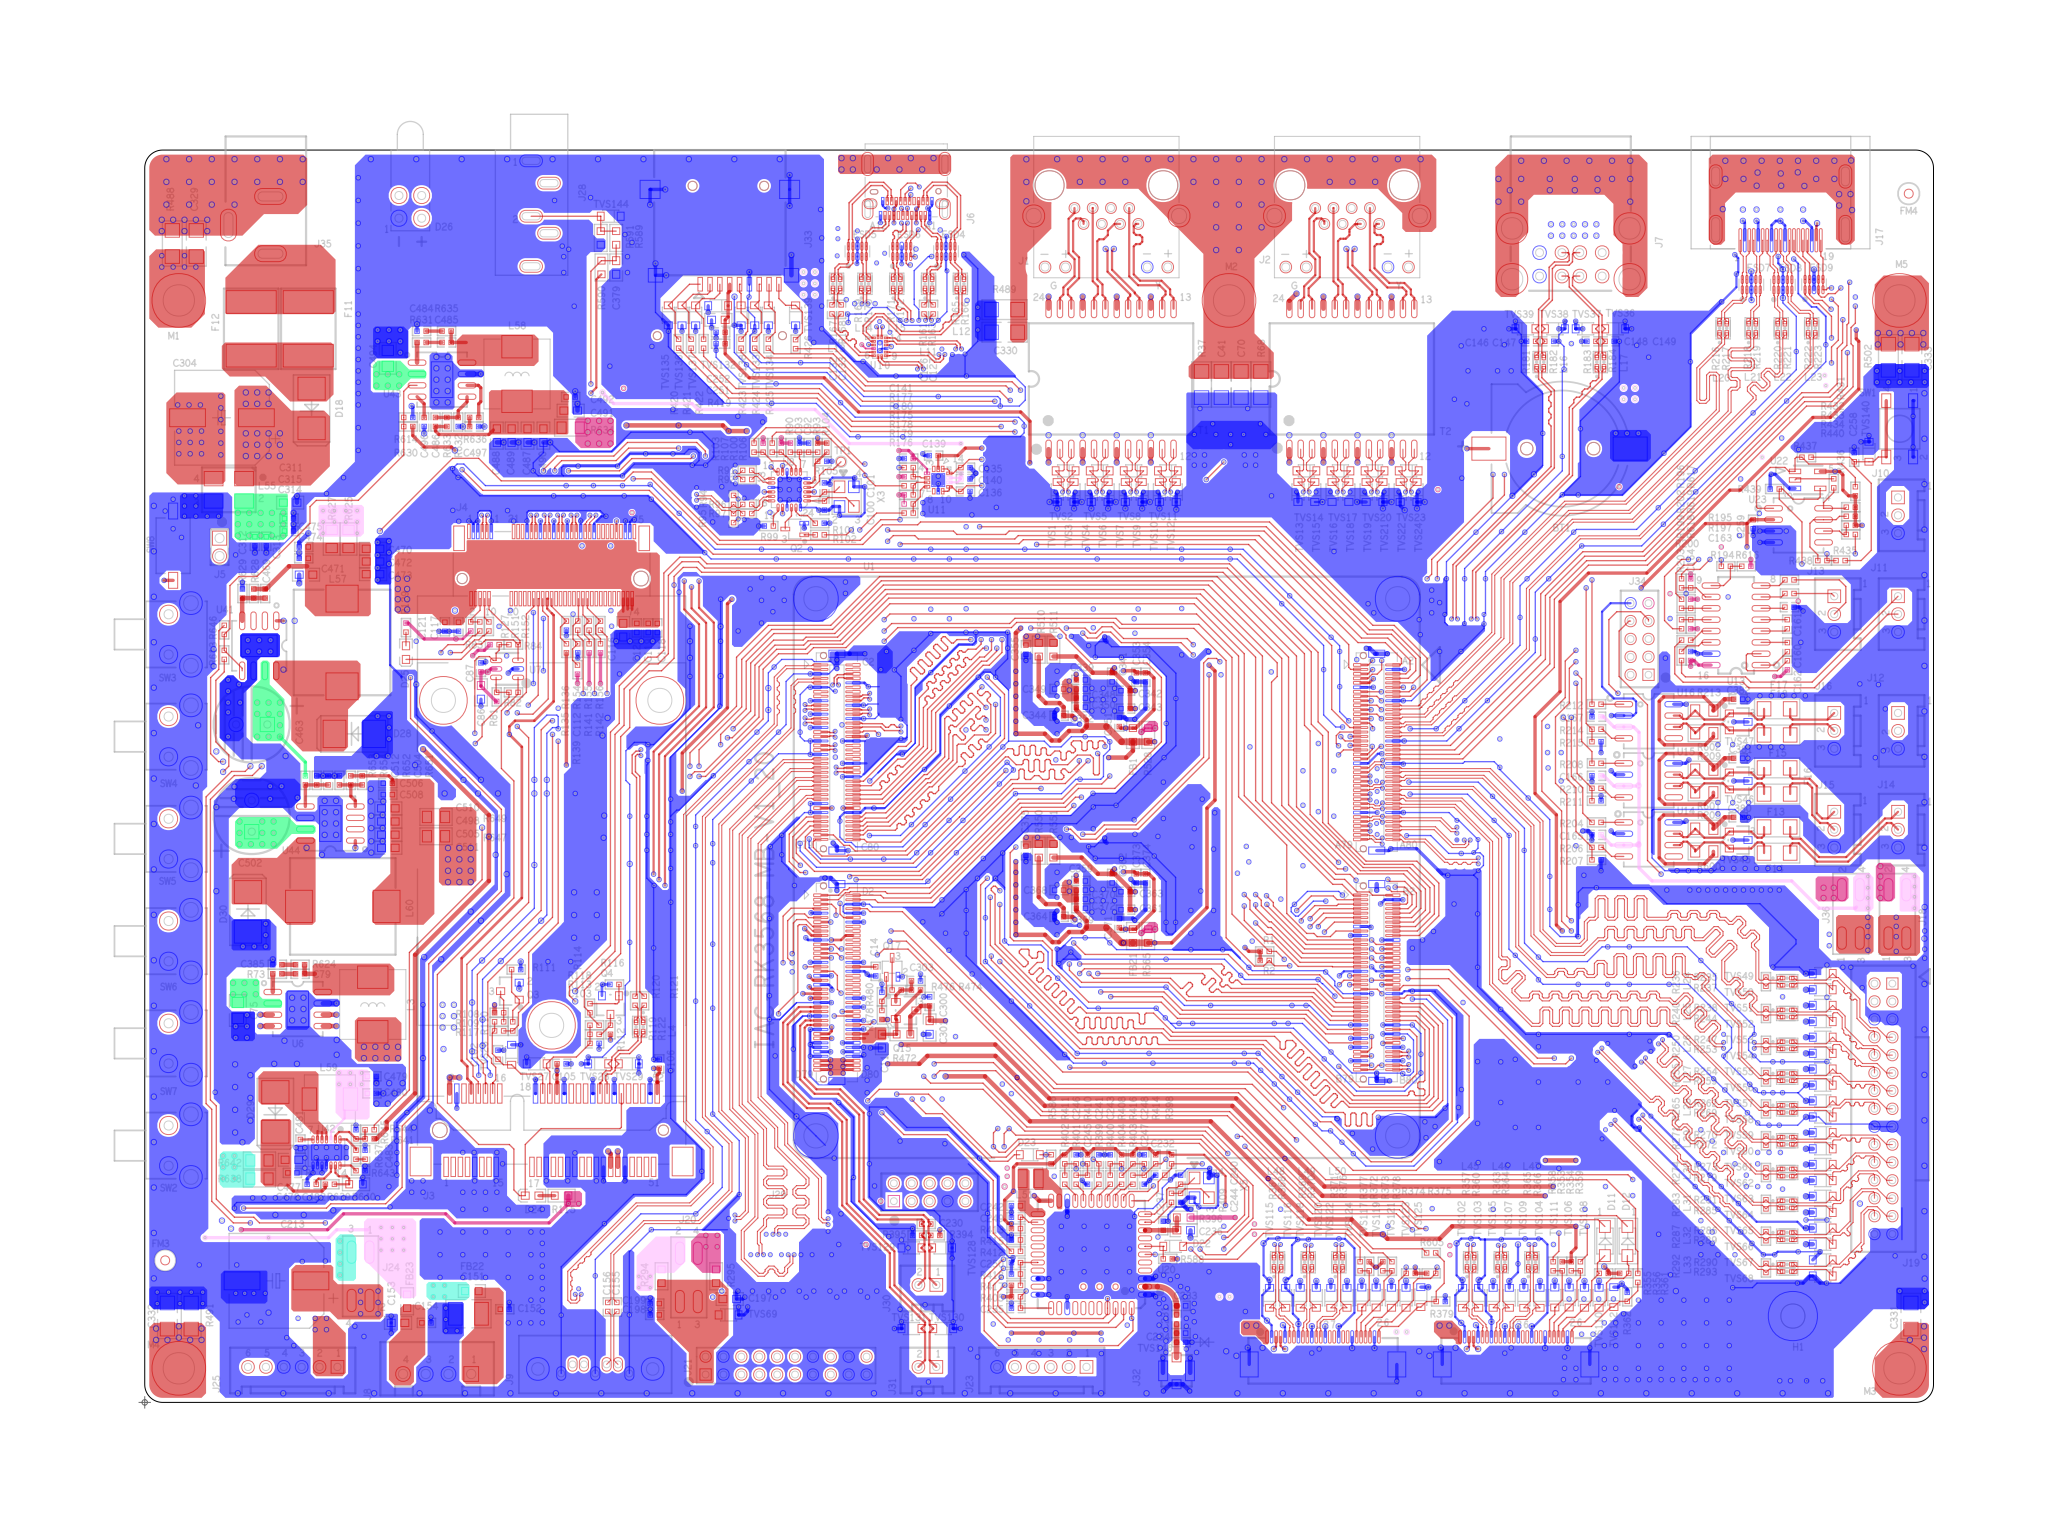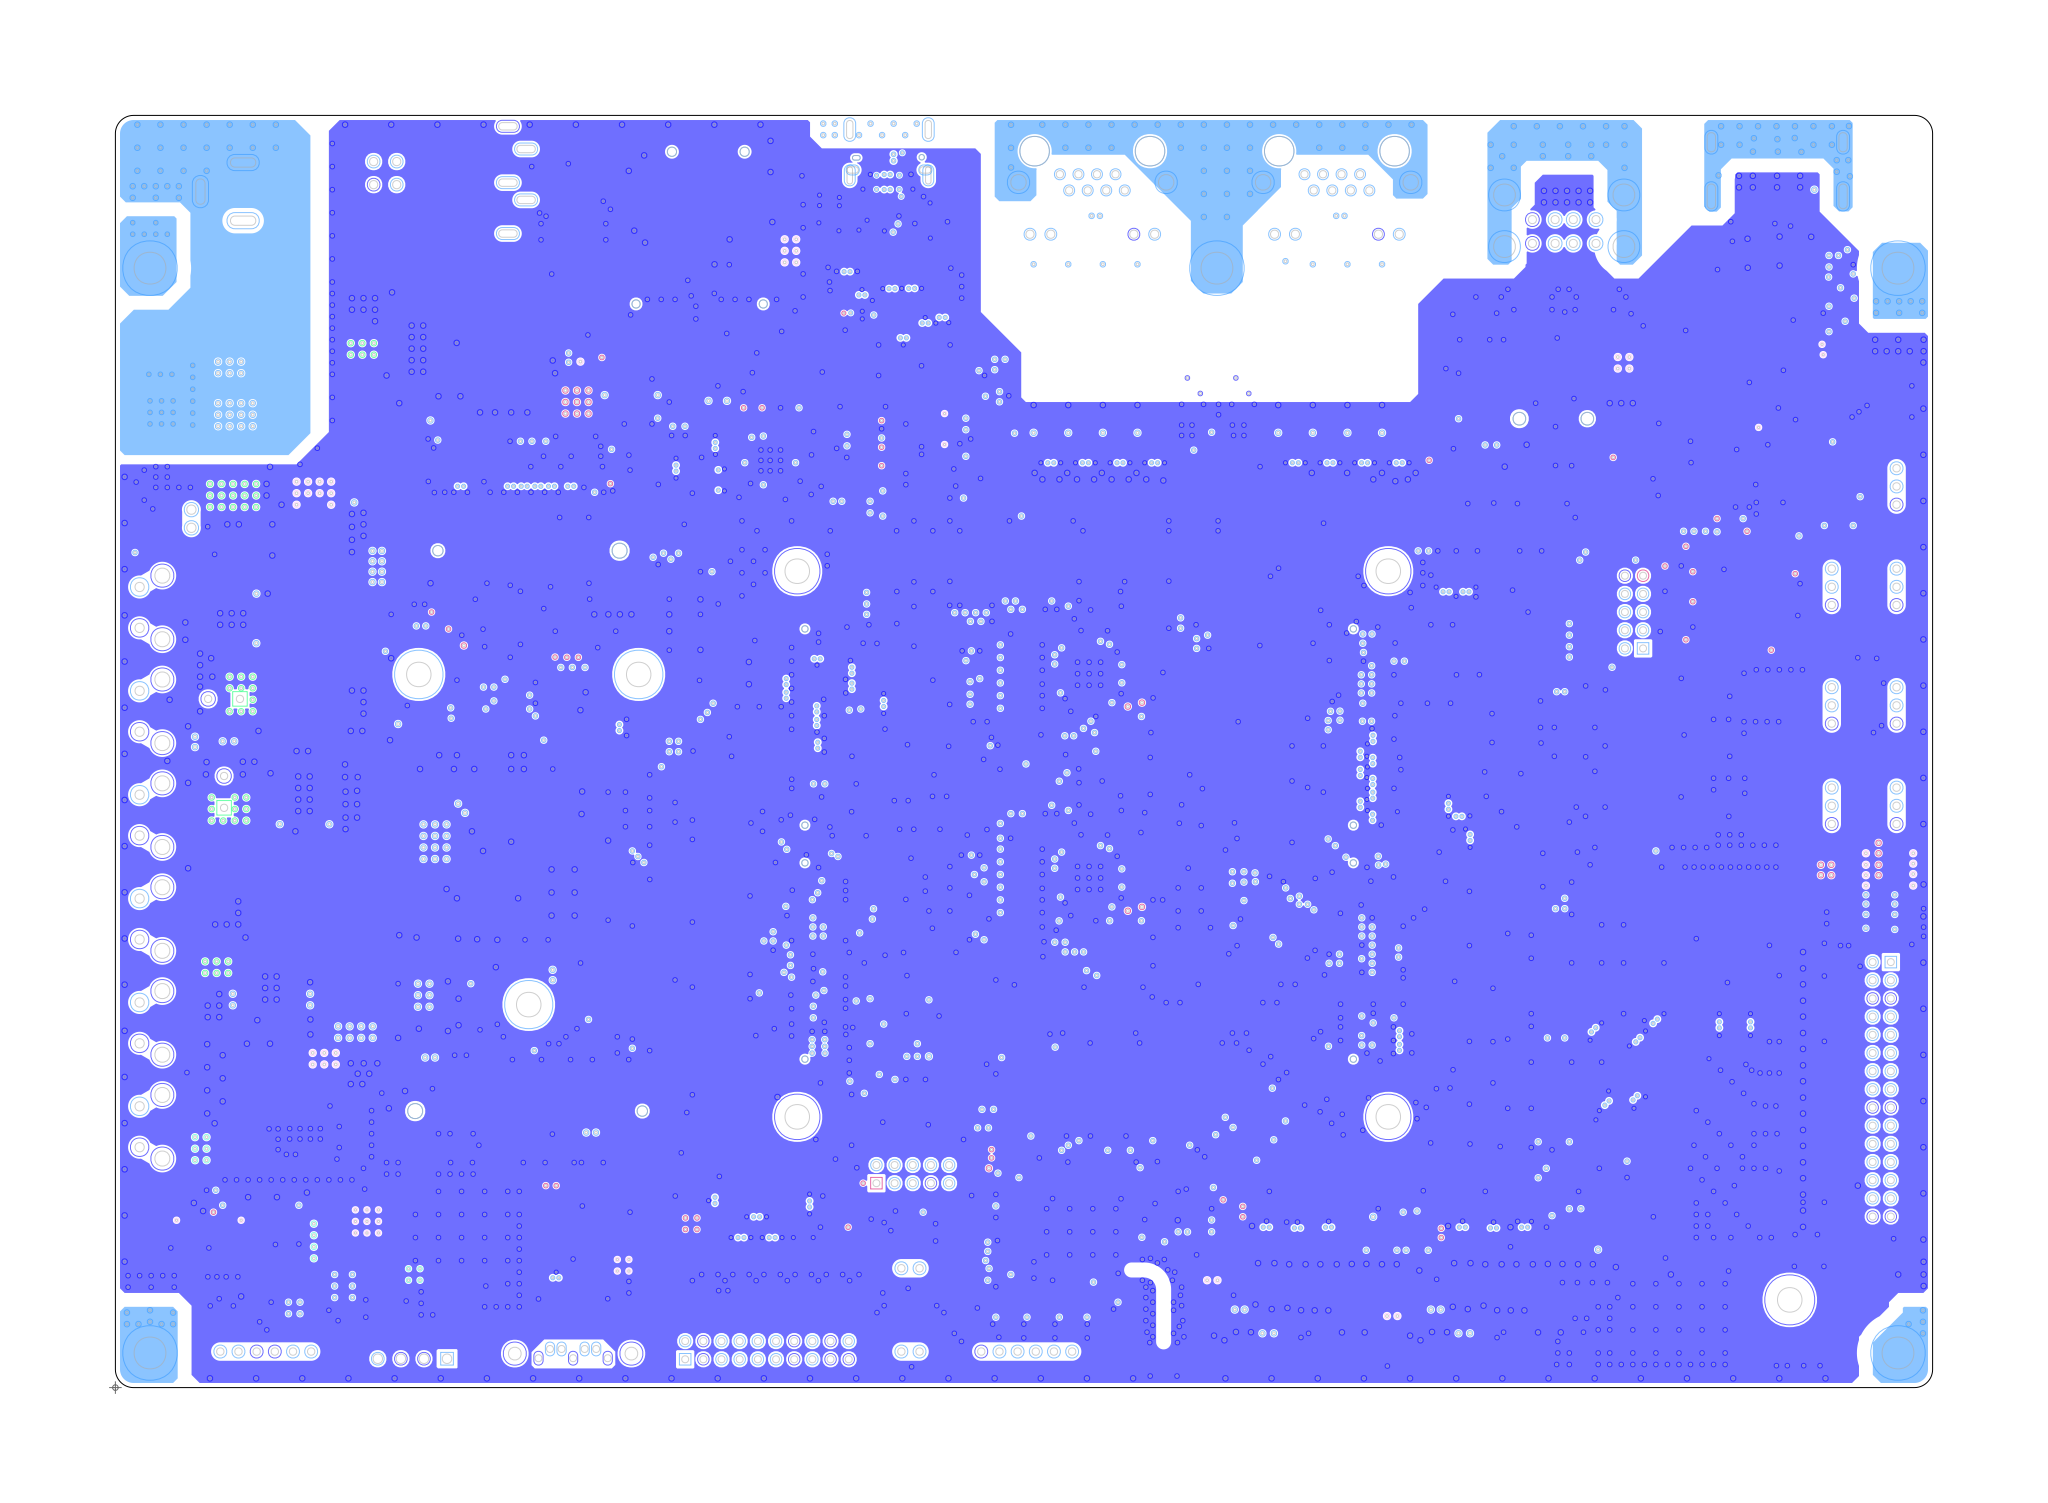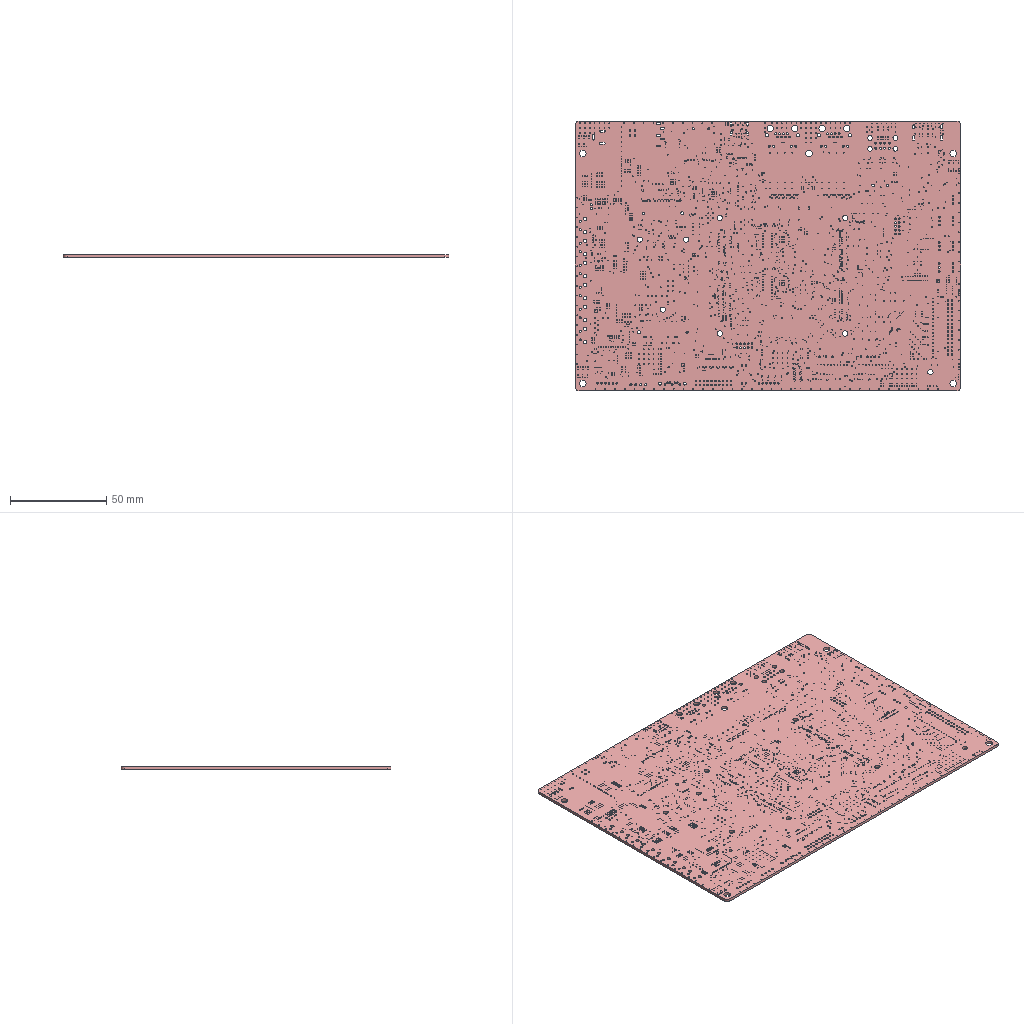Circuit board layout | Cadence Allegro | box 200 x 140 x 1.5 mm
Layer stack:
# Cadence Allegro layer stack of  (unit mm; from the constraint file cross-section; dielectric type: 0 not recorded (Allegro does not mark core vs prepreg), 3 surface material)
index,name,kind,layer,copper_thickness_mm,dielectric_type,dielectric_thickness_mm,dielectric_material,dielectric_constant
0,Top Surface,other,,,,,,
1,TOP,copper,TOP,0.0356,,,,
2,Dielectric1,dielectric,,,0,0.1016,FR-4,4.5
3,GND02,copper,GND02,0.0305,,,,
4,Dielectric2,dielectric,,,0,1.219,FR-4,4.5
5,POWER03,copper,POWER03,0.0305,,,,
6,Dielectric3,dielectric,,,0,0.1016,FR-4,4.5
7,BOTTOM,copper,BOTTOM,0.0356,,,,
8,Bottom Surface,other,,,,,,
# drill layer pairs: low layer,high layer
drill_pair,TOP,BOTTOM
Part placement, first 476 of 1143 lines:
REFDES,COMP_VALUE,SYM_NAME,SYM_X,SYM_Y,SYM_ROTATE,SYM_MIRROR
BT1,BAT1220,BAT-1220-VS,6240.970,4197.730,180.000,NO
C1,100nF/50V,SC0402,6200.000,995.158,270.000,YES
C2,100nF/50V,SC0402,6320.000,875.000,0.000,YES
C3,100nF/50V,SC0402,4700.000,770.000,180.000,YES
C4,100nF/50V,SC0402,4620.000,770.000,180.000,YES
C5,22uF/10V,SC0603,3046.000,1515.000,90.000,YES
C6,22uF/10V,SC0603,3150.000,1445.000,0.000,YES
C7,22uF/10V,SC0603,3150.000,1390.000,0.000,YES
C8,22uF/10V,SC0603,2985.000,1515.000,90.000,YES
C9,22uF/10V,SC0603,3150.000,1500.000,0.000,YES
C10,22uF/10V,SC0603,3095.000,1630.000,0.000,YES
C11,22uF/10V,SC0603,3245.000,1590.000,90.000,NO
C12,22uF/10V,SC0603,2995.000,2585.764,180.000,YES
C13,100nF/50V,SC0402,3000.000,2650.000,180.000,YES
C14,100nF/50V,SC0402,3217.709,1897.071,90.000,NO
C15,100nF/50V,SC0402,5365.000,3150.000,270.000,YES
C16,100nF/50V,SC0402,2955.000,1895.000,90.000,YES
C38,1nF/50V,SC0402,4610.000,4575.000,270.000,YES
C39,1nF/50V,SC0402,4750.000,4575.000,270.000,YES
C40,1nF/2KV,SC1206,3900.000,4831.170,270.000,YES
C41,1nF/2KV,SC1206,4739.000,4480.000,90.000,NO
C42,100nF/50V,SC0402,4428.683,4205.550,270.000,YES
C43,100nF/50V,SC0402,4278.683,4205.550,270.000,YES
C44,100nF/50V,SC0402,3978.683,4205.550,270.000,YES
C45,100nF/50V,SC0402,4128.683,4205.550,270.000,YES
C67,1nF/50V,SC0402,4820.000,4575.000,270.000,YES
C68,1nF/50V,SC0402,4960.000,4575.000,270.000,YES
C69,1nF/2KV,SC1206,5628.443,4831.170,270.000,YES
C70,1nF/2KV,SC1206,4826.000,4480.000,90.000,NO
C71,100nF/50V,SC0402,5338.443,4205.550,270.000,YES
C72,100nF/50V,SC0402,5038.443,4205.550,270.000,YES
C73,100nF/50V,SC0402,5188.443,4205.550,270.000,YES
C74,100nF/50V,SC0402,5488.443,4205.550,270.000,YES
C75,10uF/50V,SC0805,410.000,1725.000,270.000,NO
C76,10uF/50V,SC0805,410.000,1725.000,90.000,YES
C77,1nF/50V,SC0402,783.750,1756.250,0.000,YES
C78,100nF/50V,SC0402,475.000,1726.000,90.000,YES
C79,100nF/50V,SC0402,683.750,1886.250,180.000,NO
C80,100pF/50V,SC0402,763.750,1586.250,270.000,YES
C81,22uF/10V,SC0603,993.000,1435.000,90.000,YES
C82,22uF/10V,SC0603,1105.000,1435.000,90.000,YES
C83,22uF/10V,SC0603,915.000,1595.000,0.000,YES
C84,100nF/50V,SC0402,915.000,1530.000,0.000,YES
C85,100nF/50V,SC0402,573.750,1656.250,0.000,YES
C86,10uF/10V,SC0603,1480.000,3125.000,270.000,NO
C87,100nF/50V,SC0402,1480.000,3235.000,90.000,NO
C88,100nF/50V,SC0402,2670.000,4315.000,180.000,YES
C89,33pF/50V,SC0402,2490.000,4145.000,270.000,YES
C90,33pF/50V,SC0402,2440.000,4145.000,270.000,YES
C91,33pF/50V,SC0402,2385.000,4145.000,270.000,YES
C92,1uF/10V,SC0402,2922.127,4202.058,90.000,NO
C93,10nF/50V,SC0402,2882.127,4202.058,90.000,NO
C94,1uF/10V,SC0402,2852.127,3944.058,180.000,YES
C95,10nF/50V,SC0402,2842.127,4097.058,180.000,YES
C96,10nF/50V,SC0402,2772.127,3944.058,0.000,YES
C97,1uF/10V,SC0402,2772.127,3993.058,180.000,YES
C98,10nF/50V,SC0402,2985.127,4027.058,270.000,YES
C99,10nF/50V,SC0402,2772.127,4038.058,180.000,YES
C100,30pF/50V,SC0402,2992.127,3947.058,90.000,NO
C101,30pF/50V,SC0402,2992.127,4027.058,270.000,NO
C102,100nF/50V,SC0402,1555.000,1530.000,90.000,NO
C103,100nF/50V,SC0402,1980.000,1580.000,0.000,NO
C104,10uF/10V,SC0603,1345.000,1525.000,270.000,YES
C105,100nF/50V,SC0402,1835.000,1490.000,0.000,NO
C106,100nF/50V,SC0402,2265.000,1490.000,90.000,NO
C107,100nF/50V,SC0402,2085.000,1055.000,90.000,YES
C108,100nF/50V,SC0402,2035.000,1055.000,90.000,YES
C109,100nF/50V,SC0402,1405.000,1525.000,270.000,YES
C110,100nF/50V,SC0402,1656.092,3527.397,270.000,YES
C111,100nF/50V,SC0402,1696.092,3527.397,270.000,YES
C112,100nF/50V,SC0402,1906.092,3318.700,90.000,NO
C113,220nF/25V,SC0402,1916.092,3527.397,270.000,YES
C114,220nF/25V,SC0402,1956.092,3527.397,270.000,YES
C115,100nF/50V,SC0402,2101.078,3846.300,0.000,YES
C116,10uF/10V,SC0603,2106.300,3398.700,270.000,NO
C117,100nF/50V,SC0402,1381.092,3413.700,270.000,NO
C118,100nF/50V,SC0402,2256.300,3408.492,270.000,NO
C119,100nF/50V,SC0402,2216.300,3408.700,270.000,NO
C120,100nF/50V,SC0402,2166.300,3408.700,270.000,NO
C121,100nF/50V,SC0402,1321.300,3413.700,270.000,NO
C122,10uF/10V,SC0603,3338.000,4950.000,270.000,YES
C123,100nF/50V,SC0402,3405.000,4815.000,90.000,YES
C124,10uF/10V,SC0603,3471.629,5132.539,180.000,YES
C125,100nF/50V,SC0402,3465.000,5072.000,180.000,YES
C126,100nF/50V,SC0402,3430.343,4810.539,90.000,NO
C127,100nF/50V,SC0402,3470.343,4810.539,90.000,NO
C128,22uF/25V,SC0805,3295.648,5087.539,90.000,YES
C129,22uF/25V,SC0805,3221.648,5087.539,90.000,YES
C130,100nF/50V,SC0402,3365.000,5085.000,90.000,YES
C131,100nF/50V,SC0402,3000.000,5067.564,90.000,YES
C132,100nF/50V,SC0402,3025.343,4810.539,90.000,NO
C133,100nF/50V,SC0402,3065.343,4810.539,90.000,NO
C134,1nF/2KV,SC1206,3093.117,5211.300,270.000,YES
C135,220pF/50V,SC0402,3612.834,4114.183,0.000,NO
C136,220pF/50V,SC0402,3612.834,4009.183,0.000,NO
C137,4.7uF/10V,SC0402,3081.290,4695.200,270.000,YES
C138,100nF/50V,SC0402,3121.290,4695.200,270.000,YES
C139,1uF/10V,SC0402,3472.834,4167.018,180.000,NO
C140,1uF/10V,SC0402,3612.834,4064.183,0.000,NO
C141,1uF/10V,SC0402,3362.834,4154.183,180.000,NO
C142,100uF/6.3V,SC1206,6305.000,4600.000,0.000,YES
C143,1nF/50V,SC0402,6366.598,4675.125,0.000,YES
C144,100uF/6.3V,SC1206,6510.000,4600.000,180.000,YES
C145,1nF/50V,SC0402,6448.798,4675.125,180.000,YES
C146,5pF/50V,SC0402,6102.698,4670.125,180.000,NO
C147,5pF/50V,SC0402,6182.698,4670.125,0.000,NO
C148,5pF/50V,SC0402,6368.148,4670.000,180.000,NO
C149,5pF/50V,SC0402,6448.148,4670.000,0.000,NO
C150,1nF/2KV,SC1206,6245.000,5288.300,270.000,YES
C151,10uF/50V,SC1210,1425.000,390.000,180.000,NO
C152,100nF/50V,SC0402,1585.000,410.000,0.000,NO
C153,10uF/10V,SC0603,1115.000,350.000,180.000,NO
C154,100nF/50V,SC0402,1240.000,350.000,0.000,NO
C155,10nF/50V,SC0402,2078.286,420.000,270.000,NO
C156,10nF/50V,SC0402,2038.286,420.000,270.000,NO
C157,10nF/50V,SC0402,1888.286,420.000,90.000,YES
C158,10nF/50V,SC0402,1928.286,420.000,90.000,YES
C159,100nF/50V,SC0402,7020.094,3865.710,90.000,YES
C160,100nF/50V,SC0402,7230.670,3324.118,270.000,NO
C161,100nF/50V,SC0402,7230.000,3425.000,270.000,NO
C162,100nF/50V,SC0402,7230.670,3244.118,90.000,NO
C163,100nF/50V,SC0402,7240.000,3500.000,180.000,NO
C164,100nF/50V,SC0402,6805.000,3285.000,270.000,NO
C165,100nF/50V,SC0402,6390.616,2497.830,180.000,NO
C166,100nF/50V,SC0402,6390.616,2757.830,180.000,NO
C167,100nF/50V,SC0402,6390.616,3017.830,180.000,NO
C168,1nF/2KV,SC1206,7144.530,5288.300,270.000,YES
C169,1uF/10V,SC0402,7342.530,5141.300,0.000,YES
C174,10uF/10V,SC0603,7745.000,2015.000,180.000,YES
C175,100nF/50V,SC0402,7745.000,2070.000,180.000,YES
C176,100nF/50V,SC0402,7525.000,2060.000,0.000,YES
C177,100nF/50V,SC0402,7525.000,2010.000,0.000,YES
C197,10uF/10V,SC0603,2575.000,455.000,0.000,NO
C198,100nF/50V,SC0402,2245.000,385.000,180.000,NO
C199,100nF/50V,SC0402,2245.000,435.000,180.000,NO
C200,100nF/50V,SC0402,3135.000,740.000,90.000,YES
C201,100nF/50V,SC0402,3095.000,740.000,90.000,YES
C210,100nF/50V,SC0402,4298.900,330.000,270.000,YES
C211,100nF/50V,SC0402,3713.900,325.000,270.000,YES
C212,10nF/50V,SC0402,700.000,545.000,0.000,YES
C213,330uF/35V,CAP2-10P4-XX,580.000,535.000,270.000,NO
C214,22uF/25V,SC0805,890.000,290.000,180.000,YES
C215,100nF/50V,SC0402,695.000,345.000,0.000,YES
C216,10uF/10V,SC0603,5670.870,274.600,90.000,YES
C217,100nF/50V,SC0402,5610.870,274.600,90.000,YES
C218,10uF/10V,SC0603,5921.870,309.600,180.000,YES
C219,100nF/50V,SC0402,5809.130,310.400,0.000,YES
C220,10uF/10V,SC0603,4820.000,270.000,90.000,YES
C221,100nF/50V,SC0402,4820.000,380.000,270.000,YES
C222,10uF/10V,SC0603,5072.270,309.600,180.000,YES
C223,100nF/50V,SC0402,4959.530,310.400,0.000,YES
C224,47uF/16V,SC1206,1987.000,4760.300,270.000,YES
C225,47uF/16V,SC1206,2095.000,4760.300,270.000,YES
C226,10uF/10V,SC0603,2065.000,5042.700,180.000,YES
C227,10uF/10V,SC0603,1920.000,5042.700,0.000,YES
C228,100nF/50V,SC0402,3212.520,905.630,270.000,YES
C229,10uF/10V,SC0603,3090.000,1895.000,180.000,YES
C230,100pF/50V,SC0402,3440.000,785.000,180.000,NO
C231,10pF/50V,SC0402,4541.980,364.950,270.000,NO
C232,100nF/50V,SC0402,4470.000,1000.000,180.000,NO
C233,5pF/50V,SC0402,4561.980,424.950,0.000,NO
C234,5pF/50V,SC0402,4561.980,304.950,0.000,NO
C235,100nF/50V,SC0402,3835.000,415.030,180.000,NO
C236,10uF/10V,SC0603,4573.340,757.530,0.000,NO
C237,100nF/50V,SC0402,4483.340,777.530,90.000,NO
C238,4.7uF/10V,SC0402,3905.000,975.000,270.000,YES
C239,100nF/50V,SC0402,3945.000,975.000,270.000,YES
C240,24pF/50V,SC0402,4559.750,980.230,270.000,NO
C241,33pF/50V,SC0402,4200.000,1070.000,90.000,NO
C242,4.7uF/10V,SC0402,3835.000,865.000,180.000,NO
C243,33pF/50V,SC0402,4250.000,1070.000,90.000,NO
C244,24pF/50V,SC0402,4559.750,900.230,90.000,NO
C245,33pF/50V,SC0402,4150.000,980.000,270.000,NO
C246,33pF/50V,SC0402,4100.000,1070.000,90.000,NO
C247,33pF/50V,SC0402,4400.000,980.000,270.000,NO
C248,33pF/50V,SC0402,4400.000,1070.000,90.000,NO
C249,10pF/50V,SC0402,3835.000,815.000,180.000,NO
C250,1uF/10V,SC0402,3835.000,615.000,180.000,NO
C251,100nF/50V,SC0402,2535.073,4709.520,180.000,NO
C252,10uF/10V,SC0603,2525.073,4764.520,180.000,NO
C253,10uF/10V,SC0603,5730.000,4385.000,270.000,YES
C254,100nF/50V,SC0402,5795.000,4375.000,270.000,YES
C255,12pF/50V,SC0402,5935.000,4570.000,180.000,YES
C256,12pF/50V,SC0402,5845.000,4570.000,0.000,YES
C257,10uF/10V,SC0603,5767.500,4097.730,90.000,YES
C258,1nF/50V,SC0402,7525.000,4160.000,90.000,NO
C259,100nF/50V,SC0402,7080.000,3865.000,270.000,NO
C260,1nF/50V,SC0402,310.000,1315.000,270.000,YES
C261,100nF/50V,SC0402,6714.370,3497.480,90.000,YES
C300,100nF/50V,SC0402,3455.000,1765.000,90.000,NO
C301,10uF/10V,SC0603,3455.000,1650.000,270.000,NO
C303,10nF/50V,SC0402,3395.000,1855.000,0.000,NO
C304,330uF/35V,CAP2-10P4-XX,340.000,4333.700,270.000,NO
C305,100nF/50V,SC0402,385.000,4273.700,0.000,YES
C306,10nF/50V,SC0402,385.000,4222.034,0.000,YES
C307,1nF/50V,SC0402,385.000,4325.366,0.000,YES
C308,100pF/50V,SC0402,385.000,4377.032,0.000,YES
C309,10pF/50V,SC0402,385.000,4428.698,0.000,YES
C310,1uF/10V,SC0402,385.000,4170.368,0.000,YES
C311,1uF/50V,SC0603,640.000,3960.000,0.000,NO
C312,100nF/50V,SC0402,485.000,3790.000,270.000,NO
C313,1nF/50V,SC0402,535.000,3790.000,270.000,NO
C314,100pF/50V,SC0402,635.000,3835.000,0.000,NO
C315,10pF/50V,SC0402,635.000,3890.000,0.000,NO
C329,1nF/2KV,SC1206,226.850,5100.550,90.000,NO
C330,1nF/2KV,SC1206,3785.000,4710.000,180.000,NO
C331,1nF/2KV,SC1206,7774.500,380.000,90.000,NO
C332,1nF/2KV,SC1206,100.000,380.000,90.000,NO
C333,1nF/2KV,SC1206,7778.800,4600.137,270.000,NO
C334,100nF/50V,SC0402,7240.000,3495.000,180.000,YES
C335,100nF/50V,SC0402,7240.000,3545.000,0.000,YES
C336,100nF/50V,SC0402,7230.000,3425.000,270.000,YES
C337,100nF/50V,SC0402,7240.000,3345.000,0.000,YES
C338,100nF/50V,SC0402,6805.000,3575.000,270.000,YES
C339,100nF/50V,SC0402,4120.627,3179.800,0.000,NO
C340,12pF/50V,SC0402,4234.056,3327.900,270.000,YES
C341,100nF/50V,SC0402,4258.426,3191.329,270.000,NO
C342,100nF/50V,SC0402,4317.485,3132.270,180.000,NO
C343,100nF/50V,SC0402,4317.485,3053.530,180.000,NO
C344,100nF/50V,SC0402,4025.000,3022.030,180.000,NO
C345,100nF/50V,SC0402,4437.699,2837.904,0.000,YES
C346,5pF/50V,SC0402,3689.000,3217.904,0.000,YES
C347,5pF/50V,SC0402,4045.000,2857.904,90.000,YES
C348,100nF/50V,SC0402,4120.627,3139.800,0.000,NO
C349,4.7uF/10V,SC0402,4025.000,3139.800,180.000,NO
C350,100nF/50V,SC0402,4120.627,3099.800,0.000,NO
C351,100nF/50V,SC0402,4289.926,2994.471,90.000,NO
C352,4.7uF/10V,SC0402,4120.627,3059.800,180.000,NO
C353,100nF/50V,SC0402,4365.000,3191.329,270.000,NO
C354,4.7uF/10V,SC0402,4405.000,3191.329,270.000,NO
C355,4.7uF/10V,SC0402,3879.056,3312.900,270.000,NO
C356,12pF/50V,SC0402,4299.056,3327.900,90.000,YES
C357,100nF/50V,SC0402,3879.056,3312.900,90.000,YES
C359,100nF/50V,SC0402,4120.627,2294.800,0.000,NO
C360,12pF/50V,SC0402,4234.056,2442.900,270.000,YES
C361,100nF/50V,SC0402,4317.485,2168.530,180.000,NO
C362,100nF/50V,SC0402,4258.426,2306.329,270.000,NO
C363,100nF/50V,SC0402,4317.485,2247.270,180.000,NO
C364,100nF/50V,SC0402,4025.000,2137.030,180.000,NO
C365,100nF/50V,SC0402,4437.699,1952.904,0.000,YES
C366,5pF/50V,SC0402,3689.000,2332.904,0.000,YES
C367,5pF/50V,SC0402,4045.000,1972.904,90.000,YES
C368,100nF/50V,SC0402,4025.000,2254.800,180.000,NO
C369,4.7uF/10V,SC0402,4120.627,2174.800,0.000,NO
C370,100nF/50V,SC0402,4120.627,2254.800,0.000,NO
C371,100nF/50V,SC0402,4289.926,2109.471,90.000,NO
C372,4.7uF/10V,SC0402,4120.627,2214.800,180.000,NO
C373,100nF/50V,SC0402,4365.000,2306.329,270.000,NO
C374,4.7uF/10V,SC0402,4405.000,2306.329,270.000,NO
C375,4.7uF/10V,SC0402,3879.056,2427.900,270.000,NO
C376,12pF/50V,SC0402,4299.056,2442.900,90.000,YES
C377,100nF/50V,SC0402,3879.056,2427.900,90.000,YES
C379,100nF/50V,SC0603,2075.183,4995.000,270.000,NO
C380,47nF/50V,SC0402,7013.996,2575.000,0.000,NO
C381,47nF/50V,SC0402,7013.996,2835.000,0.000,NO
C382,47nF/50V,SC0402,7013.996,3095.000,0.000,NO
C383,22uF/10V,SC0603,1049.000,1435.000,90.000,YES
C384,22uF/10V,SC0603,1205.000,1550.000,180.000,YES
C385,10nF/50V,SC0402,583.750,1926.250,180.000,NO
C463,100uF/50V,EC2-3P5-08,470.862,2983.744,180.000,NO
C464,10nF/50V,SC0402,610.587,3269.844,270.000,YES
C465,10uF/50V,SC0805,440.000,3120.000,0.000,YES
C466,2.2uF/50V,SC0603,544.760,3223.744,270.000,YES
C467,2.2uF/50V,SC0603,479.760,3223.744,270.000,YES
C468,100nF/50V,SC0402,445.000,3055.000,0.000,YES
C469,82pF/50V,SC0402,530.000,3560.000,270.000,NO
C470,22uF/10V,SC0603,1005.000,3757.000,0.000,NO
C471,22uF/10V,SC0603,710.000,3643.000,180.000,NO
C472,22uF/10V,SC0603,1005.000,3701.000,0.000,NO
C473,22uF/10V,SC0603,1005.000,3645.000,0.000,NO
C474,10uF/10V,SC0402,700.000,3715.000,180.000,NO
C475,100nF/50V,SC0402,700.000,3765.000,180.000,NO
C476,10nF/50V,SC0402,660.000,3365.000,270.000,YES
C477,10uF/25V,SC0603,647.909,1067.840,0.000,NO
C478,100nF/50V,SC0402,650.000,1010.000,0.000,NO
C479,10uF/10V,SC0402,1000.000,1435.000,0.000,NO
C480,100nF/50V,SC0402,1000.000,1360.000,0.000,NO
C481,100nF/50V,SC0402,685.409,1137.091,270.000,NO
C482,33nF/50V,SC0402,735.000,960.000,180.000,NO
C483,4.7nF/50V,SC0402,970.000,1090.000,270.000,NO
C484,10nF/50V,SC0402,1218.750,4715.000,180.000,NO
C485,100nF/50V,SC0402,1328.750,4665.000,180.000,NO
C486,100pF/50V,SC0402,1280.000,4315.000,90.000,NO
C487,22uF/10V,SC0603,1685.000,4255.000,270.000,NO
C488,22uF/10V,SC0603,1550.000,4255.000,270.000,NO
C489,22uF/10V,SC0603,1615.000,4255.000,270.000,NO
C490,22uF/10V,SC0603,1755.000,4255.000,270.000,NO
C491,22uF/10V,SC0603,1875.000,4365.000,0.000,NO
C492,100nF/50V,SC0402,1875.000,4425.000,0.000,NO
C493,10uF/50V,SC0805,1070.000,4595.000,270.000,YES
C494,10uF/50V,SC0805,1070.000,4595.000,90.000,NO
C495,100nF/50V,SC0402,1145.000,4585.000,270.000,YES
C496,100nF/50V,SC0402,1230.000,4315.000,90.000,NO
C497,1nF/50V,SC0402,1450.000,4295.000,180.000,NO
C498,22uF/10V,SC0603,1072.250,2556.630,180.000,NO
C499,10uF/50V,SC0805,607.250,2611.630,270.000,YES
C500,2.2uF/50V,SC0603,710.994,2571.870,180.000,YES
C501,2.2uF/50V,SC0603,710.994,2506.870,180.000,YES
C502,100uF/50V,EC2-3P5-08,470.994,2580.768,90.000,NO
C503,100nF/50V,SC0402,542.250,2606.630,270.000,YES
C504,82pF/50V,SC0402,907.094,2737.720,270.000,NO
C505,22uF/10V,SC0603,1072.250,2498.630,180.000,NO
C506,10uF/10V,SC0402,1070.000,2725.000,180.000,NO
C507,10nF/50V,SC0402,667.250,2391.630,180.000,YES
C508,100nF/50V,SC0402,1070.000,2675.000,180.000,NO
C509,10nF/50V,SC0402,757.094,2441.043,180.000,YES
C510,22uF/10V,SC0603,1072.250,2614.630,180.000,NO
C511,22uF/10V,SC0603,1072.250,2440.630,180.000,NO
C512,10uF/10V,SC0402,807.094,2737.720,90.000,NO
D4,BZX585-B3V3,SOD-523,3080.378,5058.036,270.000,YES
D5,B5819W,SOD-123,7290.000,4475.000,0.000,YES
D6,B5819W,SOD-123,7290.000,4575.000,180.000,YES
D8,B5819W,SOD-123,3245.000,610.000,90.000,YES
D11,B5819W,SOD-123,6427.510,710.100,90.000,NO
D12,B5819W,SOD-123,6526.510,710.100,90.000,NO
D13,B5819W,SOD-123,5505.000,654.130,270.000,YES
D14,B5819W,SOD-123,5641.000,654.130,270.000,YES
D16,BAT54C,SOT23-3,5729.902,4238.730,0.000,YES
D18,SS56BG,TVS-SMB,734.500,4374.500,0.000,NO
D20,B5819W,SOD-123,4353.699,2756.800,0.000,YES
D21,B5819W,SOD-123,4353.699,1871.800,0.000,YES
D22,1N4148WS,SOD-323,4527.238,686.630,0.000,NO
D23,1N4148WS,SOD-323,3896.100,1090.000,180.000,NO
D24,YG-LED,LED0603,1705.000,910.000,0.000,NO
D25,YG-LED,LED0603,1150.000,3300.000,90.000,NO
D26,LED-1X2-R,LED4-1X2-2P54-R,1169.013,5334.241,270.000,NO
D27,BZX585-B3V3,SOD-523,6615.094,3890.710,270.000,YES
D28,SS56BG,TVS-SMB,922.759,2942.244,270.000,NO
D29,SS56BG,TVS-SMB,575.000,1278.500,0.000,NO
D30,SS56BG,TVS-SMB,454.494,2158.871,180.000,NO
ESD1,TPD4E05U06,DFN10-0P5-2P5X1P0-N,1741.300,3825.015,180.000,YES
ESD2,TPD4E05U06,DFN10-0P5-2P5X1P0-N,1861.300,3825.015,180.000,YES
ESD4,TPD4E05U06,DFN10-0P5-2P5X1P0-N,3527.123,5066.034,0.000,NO
ESD5,TPD4E05U06,DFN10-0P5-2P5X1P0-N,3137.123,5066.034,0.000,NO
ESD6,TPD4E05U06,DFN10-0P5-2P5X1P0-N,3332.123,5066.034,0.000,NO
ESD7,TPD4E05U06,DFN10-0P5-2P5X1P0-N,7072.063,4919.440,0.000,NO
ESD8,TPD4E05U06,DFN10-0P5-2P5X1P0-N,7211.063,4918.740,0.000,NO
ESD9,TPD4E05U06,DFN10-0P5-2P5X1P0-N,7348.063,4919.890,0.000,NO
F1,SMD0805-075/6V,FUSE0805,6362.500,4470.000,90.000,YES
F2,SMD0805-075/6V,FUSE0805,6452.500,4470.000,90.000,YES
F3,JK-nSMD025/16V,FUSE1206,7520.094,4041.810,0.000,YES
F4,JK-nSMD025/16V,FUSE1206,7520.094,3926.810,0.000,YES
F11,SMD0300L/16V,FUSE2920,720.000,4725.000,90.000,NO
F12,SMD0300L/16V,FUSE2920,468.700,4725.000,90.000,NO
F13,JK-nSMD025/16V,FUSE1206,7185.616,2532.500,180.000,NO
F14,JK-nSMD025/16V,FUSE1206,7185.616,2417.500,180.000,NO
F15,JK-nSMD025/16V,FUSE1206,7185.616,2792.500,180.000,NO
F16,JK-nSMD025/16V,FUSE1206,7185.616,2677.500,180.000,NO
F17,JK-nSMD025/16V,FUSE1206,7185.616,3052.500,180.000,NO
F18,JK-nSMD025/16V,FUSE1206,7185.616,2937.500,180.000,NO
FB1,120R/2A,SL0603,4349.926,2937.600,90.000,NO
FB4,120R/2A,SL0603,4610.000,4465.000,90.000,YES
FB5,120R/2A,SL0603,4750.000,4465.000,90.000,YES
FB9,120R/2A,SL0603,4820.000,4465.000,90.000,YES
FB10,120R/2A,SL0603,4960.000,4465.000,90.000,YES
FB11,120R/2A,SL0603,2847.127,4162.058,180.000,YES
FB12,120R/2A,SL0603,2727.127,4162.058,0.000,YES
FB16,120R/2A,SL0603,4238.900,340.000,90.000,YES
FB17,120R/2A,SL0603,5575.000,350.000,180.000,YES
FB18,120R/2A,SL0603,5835.400,415.870,90.000,YES
FB19,120R/2A,SL0603,4755.000,390.000,90.000,YES
FB20,120R/2A,SL0603,4985.800,415.870,90.000,YES
FB21,120R/2A,SL0603,4349.926,2052.600,90.000,NO
FB22,120R/2A,SL0603,1440.000,490.000,0.000,NO
FB23,120R/2A,SL0603,1155.000,445.000,270.000,NO
FM1,MARK,MARK,90.000,625.000,0.000,YES
FM2,MARK,MARK,7765.000,5320.000,0.000,YES
FM3,MARK,MARK,90.000,625.000,0.000,NO
FM4,MARK,MARK,7765.000,5320.000,0.000,NO
H1,M2.5X5X8,M2P5,7255.000,380.000,0.000,NO
J1,RJ45-1X1-R,RJ45-1X1-R-L,4233.103,5260.780,180.000,NO
J2,RJ45-1X1-R,RJ45-1X1-R-L,5292.863,5260.780,180.000,NO
J3,PCIE52-X2-RS,PCIE52-X2-RS-1,1791.093,1198.003,0.000,NO
J4,M2-BKEY,M2-BKEY,1791.092,3537.322,0.000,NO
J5,SIP2X1-2.0-V,SIP2X1-2P0-V,329.370,3764.370,270.000,NO
J6,USB3-1X1-TYPEC-RS,USB3-1X1-TYPEC-RS,3352.123,5330.539,180.000,NO
J7,USB2-1X2-TYPEA-R,USB2-1X2-TYPEA-R,6277.221,5232.029,180.000,NO
J8,XH4X1-2.54-V,XH4X1-2P54-V,1287.048,125.000,0.000,NO
J9,SATA-7P-1X1-V,SATA7-1P27-V,1983.268,147.283,0.000,NO
J10,PHB3X1-2.0-V,PHB3X1-2P0-V,7717.858,3904.290,90.000,NO
J11,PHB3X1-2.0-V,PHB3X1-2P0-V,7717.858,3469.330,90.000,NO
J12,PHB3X1-2.0-V,PHB3X1-2P0-V,7717.860,2955.630,90.000,NO
J13,PHB3X1-2.0-V,PHB3X1-2P0-V,7437.070,3469.330,90.000,NO
J14,PHB3X1-2.0-V,PHB3X1-2P0-V,7717.858,2520.670,90.000,NO
J15,PHB3X1-2.0-V,PHB3X1-2P0-V,7437.068,2520.670,90.000,NO
J16,PHB3X1-2.0-V,PHB3X1-2P0-V,7437.068,2955.630,90.000,NO
J17,HDMI-1X1-TYPEA-RS,HDMI-1X1-TYPEA-RS,7200.703,5278.300,180.000,NO
J18,SIP2X2-2.0-VS,SIP2X2-2P0-VS,7715.000,2150.000,0.000,NO
J19,PHB15X2-2.0-V,PHB15X2-2P0-V,7653.530,1292.220,270.000,NO
J20,SIP2X2-2.0-VS,SIP2X2-2P0-VS,2395.000,550.000,0.000,NO
J21,SIP10X2-2.0-V,SIP10X2-2P0-V,2823.189,162.048,0.000,NO
J23,PHB6X1-2.0-V,PHB6X1-2P0-V,3948.701,156.142,0.000,NO
J24,SIP2X2-2.0-VS,SIP2X2-2P0-VS,950.000,555.000,180.000,NO
J25,PHB6X1-2.0-V,PHB6X1-2P0-V,651.457,156.142,0.000,NO
J26,FPC26-X1-0.5-RS,FPC26-X1-0P5-RS-P-F,6036.377,182.838,0.000,NO
J27,FPC26-X1-0.5-RS,FPC26-X1-0P5-RS-P-F,5186.777,182.838,0.000,NO
J28,PH-JACK5-1X1-R,PH-JACK5-1X1-R,1702.833,5236.210,270.000,NO
J29,SIP5X2-2.0-V,SIP5X2-2P0-V,3455.000,925.000,0.000,NO
J30,PHB2X1-2.0-V,PHB2X1-2P0-V,3445.000,516.930,0.000,NO
J31,PHB2X1-2.0-V,PHB2X1-2P0-V,3445.000,156.142,0.000,NO
J32,IPEX-ANT4-1X1-VS,IPEX-ANT4-VS,4541.980,138.945,90.000,NO
J33,CARD-TF-PP,CARD-TF-PP,2531.343,5236.211,90.000,NO
J34,SIP5X2-2.0-V,SIP5X2-2P0-V,6580.000,3360.000,90.000,NO
J35,PWR-JACK3-1X1-R,PWR-JACK3-1X1-R,553.463,5055.660,180.000,NO
J36,SIP2X2-2.0-VS,SIP2X2-2P0-VS,7510.000,2150.000,0.000,NO
L3,10uH,IND2-06XX,1003.750,1751.250,270.000,NO
L4,90R/100M,CM4-2X1P2,2178.492,1652.443,270.000,NO
L5,90R/100M,CM4-2X1P2,1431.092,3727.557,270.000,YES
L6,90R/100M,CM4-2X1P2,1546.092,3642.557,270.000,YES
L7,90R/100M,CM4-2X1P2,1676.092,3642.557,270.000,YES
L8,90R/100M,CM4-2X1P2,1806.092,3642.557,270.000,YES
L9,90R/100M,CM4-2X1P2,1936.092,3642.557,270.000,YES
L10,90R/100M,CM4-2X1P2,2066.092,3642.557,270.000,YES
L11,90R/100M,CM4-2X1P2,3450.343,4923.339,90.000,NO
L12,90R/100M,CM4-2X1P2,3590.343,4923.339,90.000,NO
L13,90R/100M,CM4-2X1P2,3045.343,4923.339,90.000,NO
L14,90R/100M,CM4-2X1P2,3170.343,4923.339,90.000,NO
L15,90R/100M,CM4-2X1P2,3310.343,4923.339,90.000,NO
L16,90R/100M,CM4-2X1P2,6142.698,4578.585,90.000,NO
L17,90R/100M,CM4-2X1P2,6407.698,4578.585,90.000,NO
L20,90R/100M,CM4-2X1P2,6947.903,4727.250,90.000,NO
L21,90R/100M,CM4-2X1P2,7075.903,4727.250,90.000,NO
L22,90R/100M,CM4-2X1P2,7203.903,4727.250,90.000,NO
L23,90R/100M,CM4-2X1P2,7337.903,4727.250,90.000,NO
L24,90R/100M,CM4-2X1P2,7229.990,1851.660,0.000,NO
L25,90R/100M,CM4-2X1P2,7229.990,1711.660,0.000,NO
L26,90R/100M,CM4-2X1P2,7229.990,1571.660,0.000,NO
L27,220R/100M,CM4-2X1P2,7229.990,1431.660,0.000,NO
L28,90R/100M,CM4-2X1P2,7229.990,1291.660,0.000,NO
L29,90R/100M,CM4-2X1P2,7229.990,1151.660,0.000,NO
L30,90R/100M,CM4-2X1P2,7229.990,1011.660,0.000,NO
L31,90R/100M,CM4-2X1P2,7229.990,871.660,0.000,NO
L32,220R/100M,CM4-2X1P2,7229.990,731.660,0.000,NO
L33,90R/100M,CM4-2X1P2,7229.990,591.660,0.000,NO
L34,90R/100M,CM4-2X1P2,2575.687,576.155,90.000,YES
L35,90R/100M,CM4-2X1P2,2710.687,576.155,90.000,YES
L36,90R/100M,CM4-2X1P2,2845.687,576.155,90.000,YES
L37,90R/100M,CM4-2X1P2,2980.687,576.155,90.000,YES
L38,90R/100M,CM4-2X1P2,3115.687,576.155,90.000,YES
L45,220R/100M,CM4-2X1P2,5836.260,616.670,90.000,NO
L46,90R/100M,CM4-2X1P2,5971.260,616.670,90.000,NO
L47,90R/100M,CM4-2X1P2,6106.260,616.670,90.000,NO
L48,220R/100M,CM4-2X1P2,4986.660,616.670,90.000,NO
L49,90R/100M,CM4-2X1P2,5121.660,616.670,90.000,NO
L50,90R/100M,CM4-2X1P2,5256.660,616.670,90.000,NO
L51,3.3uH,IND2-2520XX,3899.740,984.765,270.000,NO
L55,500R/100M,CM4-5X5,370.185,4016.485,270.000,NO
L57,10uH,IND2-10XX,868.660,3344.569,180.000,NO
L58,10uH,IND2-06XX,1638.750,4526.250,270.000,NO
L59,6.8uH,IND2-05XX,815.000,1335.000,270.000,NO
L60,10uH,IND2-10XX,871.819,2182.970,90.000,NO
M1,CON,COPCON138,150.000,4850.004,0.000,NO
M2,CON,COPCON138,4772.985,4850.004,0.000,NO
M3,CON,COPCON138,7724.002,150.004,0.000,NO
M4,CON,COPCON138,150.000,150.000,0.000,NO
M5,CON,COPCON138,7724.002,4850.004,0.000,NO
Q1,2SK3018,SOT323-3,613.706,1566.250,270.000,YES
Q2,2SK3018,SOT323-3,2861.300,3843.958,90.000,NO
Q3,MMBT3904LT1,SOT23-3,1607.496,1810.000,90.000,NO
Q4,MMBT3904LT1,SOT23-3,2050.000,1748.500,180.000,NO
Q5,2SK3018,SOT323-3,7268.748,4806.790,270.000,YES
Q6,2SK3018,SOT323-3,7268.748,4932.918,270.000,YES
Q7,2SK3018,SOT323-3,7267.530,4681.300,270.000,YES
Q10,AO3401A,SOT23-3L,715.000,443.500,180.000,YES
Q11,2SK3018,SOT323-3,651.730,625.000,90.000,YES
Q12,2SK3018,SOT323-3,505.000,495.000,180.000,YES
Q13,2SK3018,SOT323-3,375.000,495.000,180.000,YES
Q15,AO3401A,SOT23-3L,3351.500,1725.000,270.000,NO
Q17,2SK3018,SOT323-3,3290.000,1915.000,0.000,NO
Q18,MMBT3904LT1,SOT23-3,4472.504,730.000,270.000,YES
R1,4.7K/5%,SR0402,4930.000,1985.000,180.000,NO
R2,4.7K/5%,SR0402,4930.000,1945.000,180.000,NO
R3,4.7K/5%,SR0402,6280.000,1045.000,180.000,YES
R4,4.7K/5%,SR0402,6370.000,1045.000,0.000,YES
R5,4.7K/5%,SR0402,4770.000,705.000,180.000,YES
Pad and via stacks, first 108 of 122 lines:
# Allegro (Cadence) via spans and padstacks; design units: ("mils" 3 1000)
# via spans: padstack,start_layer,end_layer,net_example,count
VAR1020,ETCH/BOTTOM,ETCH/TOP,GND,25
VAR0818,ETCH/TOP,ETCH/BOTTOM,5G_USB_D_N,243
VAR1020,ETCH/TOP,ETCH/BOTTOM,GND,1740
VAR1224,ETCH/TOP,ETCH/BOTTOM,N4118573,793
# Allegro padstack definitions: name,start_layer,end_layer,drill,plating,holeType,type
SMD35REC32,"ETCH/TOP","ETCH/TOP",0.0,"PLATED","none","smd"
SQUARE20MIL,"ETCH/TOP","ETCH/TOP",0.0,"PLATED","none","smd"
VAR1020,"ETCH/TOP","ETCH/BOTTOM",10.0,"PLATED","circle_drill","through"
SMD80OB24,"ETCH/TOP","ETCH/TOP",0.0,"PLATED","none","smd"
SMD20REC50,"ETCH/TOP","ETCH/TOP",0.0,"PLATED","none","smd"
NONPLATED45,"ETCH/TOP","ETCH/BOTTOM",45.0,"NON_PLATED","circle_drill","through"
NONPLATED65,"ETCH/TOP","ETCH/BOTTOM",65.0,"NON_PLATED","circle_drill","through"
SMD20OB50,"ETCH/TOP","ETCH/TOP",0.0,"PLATED","none","smd"
SMD16REC39,"ETCH/TOP","ETCH/TOP",0.0,"PLATED","none","smd"
SMD30REC36,"ETCH/TOP","ETCH/TOP",0.0,"PLATED","none","smd"
SMD60REC100,"ETCH/TOP","ETCH/TOP",0.0,"PLATED","none","smd"
SMD60REC63,"ETCH/TOP","ETCH/TOP",0.0,"PLATED","none","smd"
SMD40REC50,"ETCH/TOP","ETCH/TOP",0.0,"PLATED","none","smd"
SMD30REC32,"ETCH/TOP","ETCH/TOP",0.0,"PLATED","none","smd"
SMD39REC71,"ETCH/TOP","ETCH/TOP",0.0,"PLATED","none","smd"
SMD68REC68,"ETCH/TOP","ETCH/TOP",0.0,"PLATED","none","smd"
-PAD50CIR30,"ETCH/TOP","ETCH/BOTTOM",30.0,"PLATED","circle_drill","through"
-PAD50SQ30,"ETCH/TOP","ETCH/BOTTOM",30.0,"PLATED","circle_drill","through"
SMD150_102,"ETCH/TOP","ETCH/TOP",0.0,"PLATED","none","smd"
HOLE55NOPLATED,"ETCH/TOP","ETCH/BOTTOM",55.0,"NON_PLATED","circle_drill","through"
VAR1224,"ETCH/TOP","ETCH/BOTTOM",12.0,"PLATED","circle_drill","through"
MM-SMD1CIR,"ETCH/TOP","ETCH/TOP",0.0,"PLATED","none","smd"
SMD12REC64,"ETCH/TOP","ETCH/TOP",0.0,"PLATED","none","smd"
SMD48RE110,"ETCH/TOP","ETCH/TOP",0.0,"PLATED","none","smd"
SMD80REC88,"ETCH/TOP","ETCH/TOP",0.0,"NON_PLATED","none","smd"
SMD20REC60,"ETCH/TOP","ETCH/TOP",0.0,"PLATED","none","smd"
SMD85REC80,"ETCH/TOP","ETCH/TOP",0.0,"PLATED","none","smd"
NONPLATED36,"ETCH/TOP","ETCH/BOTTOM",35.43,"NON_PLATED","circle_drill","through"
SMD40X118,"ETCH/TOP","ETCH/TOP",0.0,"PLATED","none","smd"
SMD60REC40,"ETCH/TOP","ETCH/TOP",0.0,"NON_PLATED","none","smd"
SMD52REC48,"ETCH/TOP","ETCH/TOP",0.0,"PLATED","none","smd"
SMD220REC100,"ETCH/TOP","ETCH/TOP",0.0,"PLATED","none","smd"
SMD24CIR24,"ETCH/TOP","ETCH/TOP",0.0,"PLATED","none","smd"
PAD56OBL107P36X107-1,"ETCH/TOP","ETCH/BOTTOM",36.0,"PLATED","oval slot","through"
PAD56OBL103P36X83-1,"ETCH/TOP","ETCH/BOTTOM",36.0,"PLATED","oval slot","through"
SMD12OBL103,"ETCH/TOP","ETCH/TOP",0.0,"PLATED","none","smd"
PAD56CIR32P,"ETCH/TOP","ETCH/BOTTOM",32.0,"PLATED","circle_drill","through"
PAD56SQ32P,"ETCH/TOP","ETCH/BOTTOM",32.0,"PLATED","circle_drill","through"
PAD52OBL100-80CIR32,"ETCH/TOP","ETCH/BOTTOM",32.0,"PLATED","oval slot","through"
PAD140X70OB110X40P,"ETCH/TOP","ETCH/BOTTOM",40.0,"PLATED","oval slot","through"
SMD45REC50,"ETCH/TOP","ETCH/TOP",0.0,"PLATED","none","smd"
SMD110REC150,"ETCH/TOP","ETCH/TOP",0.0,"PLATED","none","smd"
SMD0P2REC0P4,"ETCH/TOP","ETCH/TOP",0.0,"PLATED","none","smd"
SMD0P55REC1P35,"ETCH/TOP","ETCH/TOP",0.0,"PLATED","none","smd"
HOLE_06TUO19,"ETCH/TOP","ETCH/BOTTOM",23.622,"PLATED","oval slot","through"
HOLED0_6-NOP,"ETCH/TOP","ETCH/BOTTOM",23.622,"NON_PLATED","circle_drill","through"
HOLE_07TUO20,"ETCH/TOP","ETCH/BOTTOM",27.559,"PLATED","oval slot","through"
SMD11REC32,"ETCH/TOP","ETCH/TOP",0.0,"PLATED","none","smd"
SMD11REC35,"ETCH/TOP","ETCH/TOP",0.0,"PLATED","none","smd"
PAD34X20-N,"ETCH/TOP","ETCH/BOTTOM",20.0,"NON_PLATED","oval slot","through"
HOLE_07TUO12,"ETCH/TOP","ETCH/BOTTOM",27.559,"PLATED","oval slot","through"
VAR0818,"ETCH/TOP","ETCH/BOTTOM",8.0,"PLATED","circle_drill","through"
SMD2P45X2P45,"ETCH/TOP","ETCH/TOP",0.0,"PLATED","none","smd"
SMD0P25X0P8,"ETCH/TOP","ETCH/TOP",0.0,"PLATED","none","smd"
SMD40CIR40,"ETCH/TOP","ETCH/TOP",0.0,"PLATED","none","smd"
SMD10OB35,"ETCH/TOP","ETCH/TOP",0.0,"PLATED","none","smd"
PAD60_40OBL30,"ETCH/TOP","ETCH/BOTTOM",30.0,"PLATED","circle_drill","through"
PAD100CIR55P,"ETCH/TOP","ETCH/BOTTOM",55.0,"PLATED","circle_drill","through"
PAD65CIR41D,"ETCH/TOP","ETCH/BOTTOM",41.0,"PLATED","circle_drill","through"
PAD65SQ41D,"ETCH/TOP","ETCH/BOTTOM",41.0,"PLATED","circle_drill","through"
SMD92RE126,"ETCH/TOP","ETCH/TOP",0.0,"PLATED","none","smd"
SMD20REC85,"ETCH/TOP","ETCH/TOP",0.0,"PLATED","none","smd"
-PAD60CIR35,"ETCH/TOP","ETCH/BOTTOM",35.0,"PLATED","circle_drill","through"
PAD80CIR40P,"ETCH/TOP","ETCH/BOTTOM",40.0,"PLATED","circle_drill","through"
PAD100CIR65P,"ETCH/TOP","ETCH/BOTTOM",65.0,"PLATED","circle_drill","through"
PAD62CIR40P,"ETCH/TOP","ETCH/BOTTOM",40.0,"PLATED","circle_drill","through"
PAD62SQ40P,"ETCH/TOP","ETCH/BOTTOM",40.0,"PLATED","circle_drill","through"
SMD70REC40,"ETCH/TOP","ETCH/TOP",0.0,"NON_PLATED","none","smd"
DRILL0P9,"ETCH/TOP","ETCH/BOTTOM",35.433,"PLATED","circle_drill","through"
SMD32RT72,"ETCH/TOP","ETCH/TOP",0.0,"PLATED","none","smd"
SMD63OL12,"ETCH/TOP","ETCH/TOP",0.0,"PLATED","none","smd"
C0P7-N,"ETCH/TOP","ETCH/BOTTOM",27.559,"NON_PLATED","circle_drill","through"
OB0P2X0P9,"ETCH/TOP","ETCH/TOP",0.0,"PLATED","none","smd"
SQ3P5,"ETCH/TOP","ETCH/TOP",0.0,"PLATED","none","smd"
OB2P4X4P0,"ETCH/TOP","ETCH/TOP",0.0,"PLATED","none","smd"
OB2P0X0P6,"ETCH/TOP","ETCH/TOP",0.0,"PLATED","none","smd"
SMD60REC22,"ETCH/TOP","ETCH/TOP",0.0,"PLATED","none","smd"
SQ1P45MM,"ETCH/TOP","ETCH/TOP",0.0,"PLATED","none","smd"
RE0P3X0P6MM,"ETCH/TOP","ETCH/TOP",0.0,"NON_PLATED","none","smd"
RE2P1X1P6,"ETCH/TOP","ETCH/TOP",0.0,"PLATED","none","smd"
RE2P5X3P4,"ETCH/TOP","ETCH/TOP",0.0,"PLATED","none","smd"
RE1P0X2P0,"ETCH/TOP","ETCH/TOP",0.0,"PLATED","none","smd"
RE3P0X3P6,"ETCH/TOP","ETCH/TOP",0.0,"NON_PLATED","none","smd"
SMD0P6X0P4,"ETCH/TOP","ETCH/TOP",0.0,"PLATED","none","smd"
C3P5D2P4,"ETCH/TOP","ETCH/BOTTOM",94.488,"PLATED","circle_drill","through"
NP40,"ETCH/TOP","ETCH/BOTTOM",40.0,"NON_PLATED","circle_drill","through"
SQ1P0,"ETCH/TOP","ETCH/TOP",0.0,"PLATED","none","smd"
RE2P2X1P0,"ETCH/TOP","ETCH/TOP",0.0,"PLATED","none","smd"
OB1P4X0P3,"ETCH/TOP","ETCH/TOP",0.0,"PLATED","none","smd"
RE2P8X2P0,"ETCH/TOP","ETCH/TOP",0.0,"PLATED","none","smd"
OB2P5X1P0,"ETCH/TOP","ETCH/TOP",0.0,"PLATED","none","smd"
D128-N,"ETCH/TOP","ETCH/BOTTOM",128.0,"NON_PLATED","circle_drill","through"
C47D31,"ETCH/TOP","ETCH/BOTTOM",31.5,"PLATED","circle_drill","through"
C51D35,"ETCH/TOP","ETCH/BOTTOM",35.44,"PLATED","circle_drill","through"
C97D67,"ETCH/TOP","ETCH/BOTTOM",67.0,"PLATED","circle_drill","through"
OB0P25X0P9,"ETCH/TOP","ETCH/TOP",0.0,"PLATED","none","smd"
OB0P4X0P9,"ETCH/TOP","ETCH/TOP",0.0,"PLATED","none","smd"
RE2P0X4P0,"ETCH/TOP","ETCH/TOP",0.0,"PLATED","none","smd"
PAD50CIR30D,"ETCH/TOP","ETCH/BOTTOM",30.0,"PLATED","circle_drill","through"
PAD50SQ30D,"ETCH/TOP","ETCH/BOTTOM",30.0,"PLATED","circle_drill","through"
RE0P6X0P8,"ETCH/TOP","ETCH/TOP",0.0,"PLATED","none","smd"